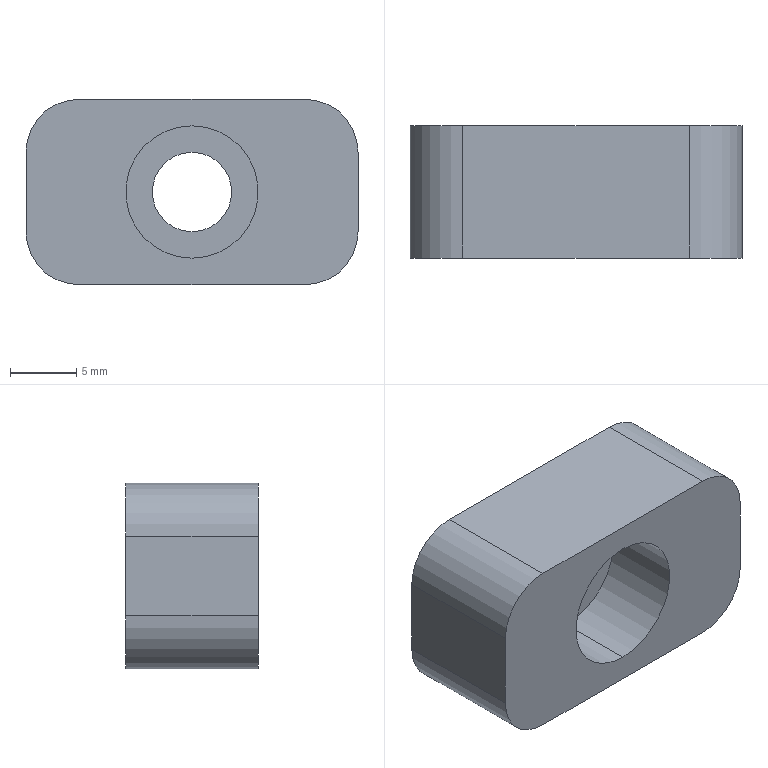Part | STEP file | 1 solid | 15 faces | box 25.075 x 10 x 14 mm | volume 2789 mm3 | cylinder 8 | plane 7 | commonest cylinder face diameters 8 x4 6 x2 10 x2
STEP:
#1=CARTESIAN_POINT('',(0.,0.,0.));
#2=DIRECTION('',(0.,0.,1.));
#3=DIRECTION('',(1.,0.,0.));
#4=AXIS2_PLACEMENT_3D('',#1,#2,#3);
#5=CARTESIAN_POINT('',(-72.862,-50.,192.673));
#6=VERTEX_POINT('',#5);
#7=CARTESIAN_POINT('',(-72.862,-44.,192.673));
#8=VERTEX_POINT('',#7);
#9=CARTESIAN_POINT('',(-72.862,-50.,192.673));
#10=DIRECTION('',(0.,1.,0.));
#11=VECTOR('',#10,1.);
#12=LINE('',#9,#11);
#13=CARTESIAN_POINT('',(-72.862,-50.,187.673));
#14=DIRECTION('',(0.,1.,0.));
#15=DIRECTION('',(0.,0.,1.));
#16=AXIS2_PLACEMENT_3D('',#13,#14,#15);
#17=CYLINDRICAL_SURFACE('',#16,5.);
#18=CARTESIAN_POINT('',(6.283,0.));
#19=DIRECTION('',(0.,1.));
#20=VECTOR('',#19,1.);
#21=LINE('',#18,#20);
#22=(GEOMETRIC_REPRESENTATION_CONTEXT(2)PARAMETRIC_REPRESENTATION_CONTEXT()REPRESENTATION_CONTEXT('',''));
#23=DEFINITIONAL_REPRESENTATION('',(#21),#22);
#24=PCURVE('',#17,#23);
#25=CARTESIAN_POINT('',(-72.862,-50.,187.673));
#26=DIRECTION('',(0.,1.,0.));
#27=DIRECTION('',(0.,0.,1.));
#28=AXIS2_PLACEMENT_3D('',#25,#26,#27);
#29=CYLINDRICAL_SURFACE('',#28,5.);
#30=CARTESIAN_POINT('',(0.,0.));
#31=DIRECTION('',(0.,1.));
#32=VECTOR('',#31,1.);
#33=LINE('',#30,#32);
#34=(GEOMETRIC_REPRESENTATION_CONTEXT(2)PARAMETRIC_REPRESENTATION_CONTEXT()REPRESENTATION_CONTEXT('',''));
#35=DEFINITIONAL_REPRESENTATION('',(#33),#34);
#36=PCURVE('',#29,#35);
#37=SURFACE_CURVE('',#12,(#24,#36),.PCURVE_S1.);
#38=EDGE_CURVE('',#6,#8,#37,.T.);
#39=ORIENTED_EDGE('',*,*,#38,.T.);
#40=CARTESIAN_POINT('',(-72.862,-44.,182.673));
#41=VERTEX_POINT('',#40);
#42=CARTESIAN_POINT('',(-72.862,-44.,187.673));
#43=DIRECTION('',(0.,-1.,0.));
#44=DIRECTION('',(0.,0.,-1.));
#45=AXIS2_PLACEMENT_3D('',#42,#43,#44);
#46=CIRCLE('',#45,5.);
#47=CARTESIAN_POINT('',(9.425,6.));
#48=DIRECTION('',(-1.,0.));
#49=VECTOR('',#48,1.);
#50=LINE('',#47,#49);
#51=(GEOMETRIC_REPRESENTATION_CONTEXT(2)PARAMETRIC_REPRESENTATION_CONTEXT()REPRESENTATION_CONTEXT('',''));
#52=DEFINITIONAL_REPRESENTATION('',(#50),#51);
#53=PCURVE('',#17,#52);
#54=CARTESIAN_POINT('',(-72.862,-44.,187.673));
#55=DIRECTION('',(0.,1.,0.));
#56=DIRECTION('',(0.,0.,1.));
#57=AXIS2_PLACEMENT_3D('',#54,#55,#56);
#58=PLANE('',#57);
#59=CARTESIAN_POINT('',(-5.,0.));
#60=CARTESIAN_POINT('',(-5.,8.66));
#61=CARTESIAN_POINT('',(2.5,4.33));
#62=CARTESIAN_POINT('',(10.,0.));
#63=CARTESIAN_POINT('',(2.5,-4.33));
#64=CARTESIAN_POINT('',(-5.,-8.66));
#65=CARTESIAN_POINT('',(-5.,0.));
#66=(BOUNDED_CURVE()B_SPLINE_CURVE(2,(#59,#60,#61,#62,#63,#64,#65),.UNSPECIFIED.,.T.,.F.)B_SPLINE_CURVE_WITH_KNOTS((1,2,2,2,2,1),(-2.094,0.,2.094,4.189,6.283,8.378),.UNSPECIFIED.)CURVE()GEOMETRIC_REPRESENTATION_ITEM()RATIONAL_B_SPLINE_CURVE((1.,0.5,1.,0.5,1.,0.5,1.))REPRESENTATION_ITEM(''));
#67=(GEOMETRIC_REPRESENTATION_CONTEXT(2)PARAMETRIC_REPRESENTATION_CONTEXT()REPRESENTATION_CONTEXT('',''));
#68=DEFINITIONAL_REPRESENTATION('',(#66),#67);
#69=PCURVE('',#58,#68);
#70=SURFACE_CURVE('',#46,(#53,#69),.PCURVE_S1.);
#71=EDGE_CURVE('',#8,#41,#70,.T.);
#72=ORIENTED_EDGE('',*,*,#71,.T.);
#73=CARTESIAN_POINT('',(-72.862,-50.,182.673));
#74=VERTEX_POINT('',#73);
#75=CARTESIAN_POINT('',(-72.862,-50.,182.673));
#76=DIRECTION('',(0.,1.,0.));
#77=VECTOR('',#76,1.);
#78=LINE('',#75,#77);
#79=CARTESIAN_POINT('',(3.142,0.));
#80=DIRECTION('',(0.,1.));
#81=VECTOR('',#80,1.);
#82=LINE('',#79,#81);
#83=(GEOMETRIC_REPRESENTATION_CONTEXT(2)PARAMETRIC_REPRESENTATION_CONTEXT()REPRESENTATION_CONTEXT('',''));
#84=DEFINITIONAL_REPRESENTATION('',(#82),#83);
#85=PCURVE('',#17,#84);
#86=CARTESIAN_POINT('',(3.142,0.));
#87=DIRECTION('',(0.,1.));
#88=VECTOR('',#87,1.);
#89=LINE('',#86,#88);
#90=(GEOMETRIC_REPRESENTATION_CONTEXT(2)PARAMETRIC_REPRESENTATION_CONTEXT()REPRESENTATION_CONTEXT('',''));
#91=DEFINITIONAL_REPRESENTATION('',(#89),#90);
#92=PCURVE('',#29,#91);
#93=SURFACE_CURVE('',#78,(#85,#92),.PCURVE_S1.);
#94=EDGE_CURVE('',#74,#41,#93,.T.);
#95=ORIENTED_EDGE('',*,*,#94,.F.);
#96=CARTESIAN_POINT('',(-72.862,-50.,187.673));
#97=DIRECTION('',(0.,1.,0.));
#98=DIRECTION('',(0.,0.,1.));
#99=AXIS2_PLACEMENT_3D('',#96,#97,#98);
#100=CIRCLE('',#99,5.);
#101=CARTESIAN_POINT('',(0.,0.));
#102=DIRECTION('',(1.,0.));
#103=VECTOR('',#102,1.);
#104=LINE('',#101,#103);
#105=(GEOMETRIC_REPRESENTATION_CONTEXT(2)PARAMETRIC_REPRESENTATION_CONTEXT()REPRESENTATION_CONTEXT('',''));
#106=DEFINITIONAL_REPRESENTATION('',(#104),#105);
#107=PCURVE('',#17,#106);
#108=CARTESIAN_POINT('',(-72.862,-50.,180.923));
#109=DIRECTION('',(0.,-1.,0.));
#110=DIRECTION('',(0.,0.,-1.));
#111=AXIS2_PLACEMENT_3D('',#108,#109,#110);
#112=PLANE('',#111);
#113=CARTESIAN_POINT('',(-11.75,0.));
#114=CARTESIAN_POINT('',(-11.75,8.66));
#115=CARTESIAN_POINT('',(-4.25,4.33));
#116=CARTESIAN_POINT('',(3.25,0.));
#117=CARTESIAN_POINT('',(-4.25,-4.33));
#118=CARTESIAN_POINT('',(-11.75,-8.66));
#119=CARTESIAN_POINT('',(-11.75,0.));
#120=(BOUNDED_CURVE()B_SPLINE_CURVE(2,(#113,#114,#115,#116,#117,#118,#119),.UNSPECIFIED.,.T.,.F.)B_SPLINE_CURVE_WITH_KNOTS((1,2,2,2,2,1),(-2.094,0.,2.094,4.189,6.283,8.378),.UNSPECIFIED.)CURVE()GEOMETRIC_REPRESENTATION_ITEM()RATIONAL_B_SPLINE_CURVE((1.,0.5,1.,0.5,1.,0.5,1.))REPRESENTATION_ITEM(''));
#121=(GEOMETRIC_REPRESENTATION_CONTEXT(2)PARAMETRIC_REPRESENTATION_CONTEXT()REPRESENTATION_CONTEXT('',''));
#122=DEFINITIONAL_REPRESENTATION('',(#120),#121);
#123=PCURVE('',#112,#122);
#124=SURFACE_CURVE('',#100,(#107,#123),.PCURVE_S1.);
#125=EDGE_CURVE('',#74,#6,#124,.T.);
#126=ORIENTED_EDGE('',*,*,#125,.T.);
#127=EDGE_LOOP('',(#39,#72,#95,#126));
#128=FACE_BOUND('',#127,.F.);
#129=ADVANCED_FACE('',(#128),#17,.F.);
#130=CARTESIAN_POINT('',(-72.862,-44.,190.673));
#131=VERTEX_POINT('',#130);
#132=CARTESIAN_POINT('',(-72.862,-40.,190.673));
#133=VERTEX_POINT('',#132);
#134=CARTESIAN_POINT('',(-72.862,-50.,190.673));
#135=DIRECTION('',(0.,1.,0.));
#136=VECTOR('',#135,1.);
#137=LINE('',#134,#136);
#138=CARTESIAN_POINT('',(-72.862,-50.,187.673));
#139=DIRECTION('',(0.,1.,0.));
#140=DIRECTION('',(0.,0.,1.));
#141=AXIS2_PLACEMENT_3D('',#138,#139,#140);
#142=CYLINDRICAL_SURFACE('',#141,3.);
#143=CARTESIAN_POINT('',(6.283,0.));
#144=DIRECTION('',(0.,1.));
#145=VECTOR('',#144,1.);
#146=LINE('',#143,#145);
#147=(GEOMETRIC_REPRESENTATION_CONTEXT(2)PARAMETRIC_REPRESENTATION_CONTEXT()REPRESENTATION_CONTEXT('',''));
#148=DEFINITIONAL_REPRESENTATION('',(#146),#147);
#149=PCURVE('',#142,#148);
#150=CARTESIAN_POINT('',(-72.862,-50.,187.673));
#151=DIRECTION('',(0.,1.,0.));
#152=DIRECTION('',(0.,0.,1.));
#153=AXIS2_PLACEMENT_3D('',#150,#151,#152);
#154=CYLINDRICAL_SURFACE('',#153,3.);
#155=CARTESIAN_POINT('',(0.,0.));
#156=DIRECTION('',(0.,1.));
#157=VECTOR('',#156,1.);
#158=LINE('',#155,#157);
#159=(GEOMETRIC_REPRESENTATION_CONTEXT(2)PARAMETRIC_REPRESENTATION_CONTEXT()REPRESENTATION_CONTEXT('',''));
#160=DEFINITIONAL_REPRESENTATION('',(#158),#159);
#161=PCURVE('',#154,#160);
#162=SURFACE_CURVE('',#137,(#149,#161),.PCURVE_S1.);
#163=EDGE_CURVE('',#131,#133,#162,.T.);
#164=ORIENTED_EDGE('',*,*,#163,.T.);
#165=CARTESIAN_POINT('',(-72.862,-40.,184.673));
#166=VERTEX_POINT('',#165);
#167=CARTESIAN_POINT('',(-72.862,-40.,187.673));
#168=DIRECTION('',(0.,-1.,0.));
#169=DIRECTION('',(0.,0.,-1.));
#170=AXIS2_PLACEMENT_3D('',#167,#168,#169);
#171=CIRCLE('',#170,3.);
#172=CARTESIAN_POINT('',(9.425,10.));
#173=DIRECTION('',(-1.,0.));
#174=VECTOR('',#173,1.);
#175=LINE('',#172,#174);
#176=(GEOMETRIC_REPRESENTATION_CONTEXT(2)PARAMETRIC_REPRESENTATION_CONTEXT()REPRESENTATION_CONTEXT('',''));
#177=DEFINITIONAL_REPRESENTATION('',(#175),#176);
#178=PCURVE('',#142,#177);
#179=CARTESIAN_POINT('',(-72.862,-40.,187.923));
#180=DIRECTION('',(0.,-1.,0.));
#181=DIRECTION('',(0.,0.,-1.));
#182=AXIS2_PLACEMENT_3D('',#179,#180,#181);
#183=PLANE('',#182);
#184=CARTESIAN_POINT('',(0.25,0.));
#185=DIRECTION('',(1.,0.));
#186=AXIS2_PLACEMENT_2D('',#184,#185);
#187=CIRCLE('',#186,3.);
#188=(GEOMETRIC_REPRESENTATION_CONTEXT(2)PARAMETRIC_REPRESENTATION_CONTEXT()REPRESENTATION_CONTEXT('',''));
#189=DEFINITIONAL_REPRESENTATION('',(#187),#188);
#190=PCURVE('',#183,#189);
#191=SURFACE_CURVE('',#171,(#178,#190),.PCURVE_S1.);
#192=EDGE_CURVE('',#133,#166,#191,.T.);
#193=ORIENTED_EDGE('',*,*,#192,.T.);
#194=CARTESIAN_POINT('',(-72.862,-44.,184.673));
#195=VERTEX_POINT('',#194);
#196=CARTESIAN_POINT('',(-72.862,-50.,184.673));
#197=DIRECTION('',(0.,1.,0.));
#198=VECTOR('',#197,1.);
#199=LINE('',#196,#198);
#200=CARTESIAN_POINT('',(3.142,0.));
#201=DIRECTION('',(0.,1.));
#202=VECTOR('',#201,1.);
#203=LINE('',#200,#202);
#204=(GEOMETRIC_REPRESENTATION_CONTEXT(2)PARAMETRIC_REPRESENTATION_CONTEXT()REPRESENTATION_CONTEXT('',''));
#205=DEFINITIONAL_REPRESENTATION('',(#203),#204);
#206=PCURVE('',#142,#205);
#207=CARTESIAN_POINT('',(3.142,0.));
#208=DIRECTION('',(0.,1.));
#209=VECTOR('',#208,1.);
#210=LINE('',#207,#209);
#211=(GEOMETRIC_REPRESENTATION_CONTEXT(2)PARAMETRIC_REPRESENTATION_CONTEXT()REPRESENTATION_CONTEXT('',''));
#212=DEFINITIONAL_REPRESENTATION('',(#210),#211);
#213=PCURVE('',#154,#212);
#214=SURFACE_CURVE('',#199,(#206,#213),.PCURVE_S1.);
#215=EDGE_CURVE('',#195,#166,#214,.T.);
#216=ORIENTED_EDGE('',*,*,#215,.F.);
#217=CARTESIAN_POINT('',(-72.862,-44.,187.673));
#218=DIRECTION('',(0.,-1.,0.));
#219=DIRECTION('',(0.,0.,1.));
#220=AXIS2_PLACEMENT_3D('',#217,#218,#219);
#221=CIRCLE('',#220,3.);
#222=CARTESIAN_POINT('',(6.283,6.));
#223=DIRECTION('',(-1.,0.));
#224=VECTOR('',#223,1.);
#225=LINE('',#222,#224);
#226=(GEOMETRIC_REPRESENTATION_CONTEXT(2)PARAMETRIC_REPRESENTATION_CONTEXT()REPRESENTATION_CONTEXT('',''));
#227=DEFINITIONAL_REPRESENTATION('',(#225),#226);
#228=PCURVE('',#142,#227);
#229=CARTESIAN_POINT('',(3.,0.));
#230=CARTESIAN_POINT('',(3.,-5.196));
#231=CARTESIAN_POINT('',(-1.5,-2.598));
#232=CARTESIAN_POINT('',(-6.,0.));
#233=CARTESIAN_POINT('',(-1.5,2.598));
#234=CARTESIAN_POINT('',(3.,5.196));
#235=CARTESIAN_POINT('',(3.,0.));
#236=(BOUNDED_CURVE()B_SPLINE_CURVE(2,(#229,#230,#231,#232,#233,#234,#235),.UNSPECIFIED.,.T.,.F.)B_SPLINE_CURVE_WITH_KNOTS((1,2,2,2,2,1),(-2.094,0.,2.094,4.189,6.283,8.378),.UNSPECIFIED.)CURVE()GEOMETRIC_REPRESENTATION_ITEM()RATIONAL_B_SPLINE_CURVE((1.,0.5,1.,0.5,1.,0.5,1.))REPRESENTATION_ITEM(''));
#237=(GEOMETRIC_REPRESENTATION_CONTEXT(2)PARAMETRIC_REPRESENTATION_CONTEXT()REPRESENTATION_CONTEXT('',''));
#238=DEFINITIONAL_REPRESENTATION('',(#236),#237);
#239=PCURVE('',#58,#238);
#240=SURFACE_CURVE('',#221,(#228,#239),.PCURVE_S1.);
#241=EDGE_CURVE('',#131,#195,#240,.T.);
#242=ORIENTED_EDGE('',*,*,#241,.F.);
#243=EDGE_LOOP('',(#164,#193,#216,#242));
#244=FACE_BOUND('',#243,.F.);
#245=ADVANCED_FACE('',(#244),#142,.F.);
#246=CARTESIAN_POINT('',(-81.4,-50.,180.673));
#247=VERTEX_POINT('',#246);
#248=CARTESIAN_POINT('',(-64.325,-50.,180.673));
#249=VERTEX_POINT('',#248);
#250=CARTESIAN_POINT('',(-72.862,-50.,180.673));
#251=DIRECTION('',(1.,0.,0.));
#252=VECTOR('',#251,1.);
#253=LINE('',#250,#252);
#254=CARTESIAN_POINT('',(-72.862,-42.,180.673));
#255=DIRECTION('',(0.,0.,-1.));
#256=DIRECTION('',(-1.,0.,0.));
#257=AXIS2_PLACEMENT_3D('',#254,#255,#256);
#258=PLANE('',#257);
#259=CARTESIAN_POINT('',(0.,-8.));
#260=DIRECTION('',(-1.,0.));
#261=VECTOR('',#260,1.);
#262=LINE('',#259,#261);
#263=(GEOMETRIC_REPRESENTATION_CONTEXT(2)PARAMETRIC_REPRESENTATION_CONTEXT()REPRESENTATION_CONTEXT('',''));
#264=DEFINITIONAL_REPRESENTATION('',(#262),#263);
#265=PCURVE('',#258,#264);
#266=CARTESIAN_POINT('',(0.25,0.));
#267=DIRECTION('',(0.,1.));
#268=VECTOR('',#267,1.);
#269=LINE('',#266,#268);
#270=(GEOMETRIC_REPRESENTATION_CONTEXT(2)PARAMETRIC_REPRESENTATION_CONTEXT()REPRESENTATION_CONTEXT('',''));
#271=DEFINITIONAL_REPRESENTATION('',(#269),#270);
#272=PCURVE('',#112,#271);
#273=SURFACE_CURVE('',#253,(#265,#272),.PCURVE_S1.);
#274=EDGE_CURVE('',#247,#249,#273,.T.);
#275=ORIENTED_EDGE('',*,*,#274,.F.);
#276=CARTESIAN_POINT('',(-81.4,-40.,180.673));
#277=VERTEX_POINT('',#276);
#278=CARTESIAN_POINT('',(-81.4,-42.,180.673));
#279=DIRECTION('',(0.,1.,0.));
#280=VECTOR('',#279,1.);
#281=LINE('',#278,#280);
#282=CARTESIAN_POINT('',(8.537,0.));
#283=DIRECTION('',(0.,1.));
#284=VECTOR('',#283,1.);
#285=LINE('',#282,#284);
#286=(GEOMETRIC_REPRESENTATION_CONTEXT(2)PARAMETRIC_REPRESENTATION_CONTEXT()REPRESENTATION_CONTEXT('',''));
#287=DEFINITIONAL_REPRESENTATION('',(#285),#286);
#288=PCURVE('',#258,#287);
#289=CARTESIAN_POINT('',(-81.4,-42.,184.673));
#290=DIRECTION('',(0.,-1.,0.));
#291=DIRECTION('',(0.,0.,-1.));
#292=AXIS2_PLACEMENT_3D('',#289,#290,#291);
#293=CYLINDRICAL_SURFACE('',#292,4.);
#294=CARTESIAN_POINT('',(6.283,0.));
#295=DIRECTION('',(0.,-1.));
#296=VECTOR('',#295,1.);
#297=LINE('',#294,#296);
#298=(GEOMETRIC_REPRESENTATION_CONTEXT(2)PARAMETRIC_REPRESENTATION_CONTEXT()REPRESENTATION_CONTEXT('',''));
#299=DEFINITIONAL_REPRESENTATION('',(#297),#298);
#300=PCURVE('',#293,#299);
#301=SURFACE_CURVE('',#281,(#288,#300),.PCURVE_S1.);
#302=EDGE_CURVE('',#247,#277,#301,.T.);
#303=ORIENTED_EDGE('',*,*,#302,.T.);
#304=CARTESIAN_POINT('',(-64.325,-40.,180.673));
#305=VERTEX_POINT('',#304);
#306=CARTESIAN_POINT('',(-72.862,-40.,180.673));
#307=DIRECTION('',(-1.,0.,0.));
#308=VECTOR('',#307,1.);
#309=LINE('',#306,#308);
#310=CARTESIAN_POINT('',(0.,2.));
#311=DIRECTION('',(1.,0.));
#312=VECTOR('',#311,1.);
#313=LINE('',#310,#312);
#314=(GEOMETRIC_REPRESENTATION_CONTEXT(2)PARAMETRIC_REPRESENTATION_CONTEXT()REPRESENTATION_CONTEXT('',''));
#315=DEFINITIONAL_REPRESENTATION('',(#313),#314);
#316=PCURVE('',#258,#315);
#317=CARTESIAN_POINT('',(7.25,0.));
#318=DIRECTION('',(0.,-1.));
#319=VECTOR('',#318,1.);
#320=LINE('',#317,#319);
#321=(GEOMETRIC_REPRESENTATION_CONTEXT(2)PARAMETRIC_REPRESENTATION_CONTEXT()REPRESENTATION_CONTEXT('',''));
#322=DEFINITIONAL_REPRESENTATION('',(#320),#321);
#323=PCURVE('',#183,#322);
#324=SURFACE_CURVE('',#309,(#316,#323),.PCURVE_S1.);
#325=EDGE_CURVE('',#305,#277,#324,.T.);
#326=ORIENTED_EDGE('',*,*,#325,.F.);
#327=CARTESIAN_POINT('',(-64.325,-42.,180.673));
#328=DIRECTION('',(0.,-1.,0.));
#329=VECTOR('',#328,1.);
#330=LINE('',#327,#329);
#331=CARTESIAN_POINT('',(-8.537,0.));
#332=DIRECTION('',(0.,-1.));
#333=VECTOR('',#332,1.);
#334=LINE('',#331,#333);
#335=(GEOMETRIC_REPRESENTATION_CONTEXT(2)PARAMETRIC_REPRESENTATION_CONTEXT()REPRESENTATION_CONTEXT('',''));
#336=DEFINITIONAL_REPRESENTATION('',(#334),#335);
#337=PCURVE('',#258,#336);
#338=CARTESIAN_POINT('',(-64.325,-42.,184.673));
#339=DIRECTION('',(0.,1.,0.));
#340=DIRECTION('',(0.,0.,1.));
#341=AXIS2_PLACEMENT_3D('',#338,#339,#340);
#342=CYLINDRICAL_SURFACE('',#341,4.);
#343=CARTESIAN_POINT('',(3.142,0.));
#344=DIRECTION('',(0.,-1.));
#345=VECTOR('',#344,1.);
#346=LINE('',#343,#345);
#347=(GEOMETRIC_REPRESENTATION_CONTEXT(2)PARAMETRIC_REPRESENTATION_CONTEXT()REPRESENTATION_CONTEXT('',''));
#348=DEFINITIONAL_REPRESENTATION('',(#346),#347);
#349=PCURVE('',#342,#348);
#350=SURFACE_CURVE('',#330,(#337,#349),.PCURVE_S1.);
#351=EDGE_CURVE('',#305,#249,#350,.T.);
#352=ORIENTED_EDGE('',*,*,#351,.T.);
#353=EDGE_LOOP('',(#275,#303,#326,#352));
#354=FACE_BOUND('',#353,.T.);
#355=ADVANCED_FACE('',(#354),#258,.T.);
#356=ORIENTED_EDGE('',*,*,#192,.T.);
#357=CARTESIAN_POINT('',(-72.862,-40.,187.673));
#358=DIRECTION('',(0.,-1.,0.));
#359=DIRECTION('',(0.,0.,-1.));
#360=AXIS2_PLACEMENT_3D('',#357,#358,#359);
#361=CIRCLE('',#360,3.);
#362=CARTESIAN_POINT('',(0.25,0.));
#363=DIRECTION('',(1.,0.));
#364=AXIS2_PLACEMENT_2D('',#362,#363);
#365=CIRCLE('',#364,3.);
#366=(GEOMETRIC_REPRESENTATION_CONTEXT(2)PARAMETRIC_REPRESENTATION_CONTEXT()REPRESENTATION_CONTEXT('',''));
#367=DEFINITIONAL_REPRESENTATION('',(#365),#366);
#368=PCURVE('',#183,#367);
#369=CARTESIAN_POINT('',(3.142,10.));
#370=DIRECTION('',(-1.,0.));
#371=VECTOR('',#370,1.);
#372=LINE('',#369,#371);
#373=(GEOMETRIC_REPRESENTATION_CONTEXT(2)PARAMETRIC_REPRESENTATION_CONTEXT()REPRESENTATION_CONTEXT('',''));
#374=DEFINITIONAL_REPRESENTATION('',(#372),#373);
#375=PCURVE('',#154,#374);
#376=SURFACE_CURVE('',#361,(#368,#375),.PCURVE_S1.);
#377=EDGE_CURVE('',#166,#133,#376,.T.);
#378=ORIENTED_EDGE('',*,*,#377,.T.);
#379=EDGE_LOOP('',(#356,#378));
#380=FACE_BOUND('',#379,.T.);
#381=ORIENTED_EDGE('',*,*,#325,.T.);
#382=CARTESIAN_POINT('',(-85.4,-40.,184.673));
#383=VERTEX_POINT('',#382);
#384=CARTESIAN_POINT('',(-81.4,-40.,184.673));
#385=DIRECTION('',(0.,1.,0.));
#386=DIRECTION('',(0.,0.,-1.));
#387=AXIS2_PLACEMENT_3D('',#384,#385,#386);
#388=CIRCLE('',#387,4.);
#389=CARTESIAN_POINT('',(7.25,-8.537));
#390=CARTESIAN_POINT('',(7.25,-15.466));
#391=CARTESIAN_POINT('',(1.25,-12.002));
#392=CARTESIAN_POINT('',(-4.75,-8.537));
#393=CARTESIAN_POINT('',(1.25,-5.073));
#394=CARTESIAN_POINT('',(7.25,-1.609));
#395=CARTESIAN_POINT('',(7.25,-8.537));
#396=(BOUNDED_CURVE()B_SPLINE_CURVE(2,(#389,#390,#391,#392,#393,#394,#395),.UNSPECIFIED.,.T.,.F.)B_SPLINE_CURVE_WITH_KNOTS((1,2,2,2,2,1),(-2.094,0.,2.094,4.189,6.283,8.378),.UNSPECIFIED.)CURVE()GEOMETRIC_REPRESENTATION_ITEM()RATIONAL_B_SPLINE_CURVE((1.,0.5,1.,0.5,1.,0.5,1.))REPRESENTATION_ITEM(''));
#397=(GEOMETRIC_REPRESENTATION_CONTEXT(2)PARAMETRIC_REPRESENTATION_CONTEXT()REPRESENTATION_CONTEXT('',''));
#398=DEFINITIONAL_REPRESENTATION('',(#396),#397);
#399=PCURVE('',#183,#398);
#400=CARTESIAN_POINT('',(6.283,-2.));
#401=DIRECTION('',(-1.,0.));
#402=VECTOR('',#401,1.);
#403=LINE('',#400,#402);
#404=(GEOMETRIC_REPRESENTATION_CONTEXT(2)PARAMETRIC_REPRESENTATION_CONTEXT()REPRESENTATION_CONTEXT('',''));
#405=DEFINITIONAL_REPRESENTATION('',(#403),#404);
#406=PCURVE('',#293,#405);
#407=SURFACE_CURVE('',#388,(#399,#406),.PCURVE_S1.);
#408=EDGE_CURVE('',#277,#383,#407,.T.);
#409=ORIENTED_EDGE('',*,*,#408,.T.);
#410=CARTESIAN_POINT('',(-85.4,-40.,190.673));
#411=VERTEX_POINT('',#410);
#412=CARTESIAN_POINT('',(-85.4,-40.,180.923));
#413=DIRECTION('',(0.,0.,1.));
#414=VECTOR('',#413,1.);
#415=LINE('',#412,#414);
#416=CARTESIAN_POINT('',(7.,-12.537));
#417=DIRECTION('',(-1.,0.));
#418=VECTOR('',#417,1.);
#419=LINE('',#416,#418);
#420=(GEOMETRIC_REPRESENTATION_CONTEXT(2)PARAMETRIC_REPRESENTATION_CONTEXT()REPRESENTATION_CONTEXT('',''));
#421=DEFINITIONAL_REPRESENTATION('',(#419),#420);
#422=PCURVE('',#183,#421);
#423=CARTESIAN_POINT('',(-85.4,-42.,180.923));
#424=DIRECTION('',(-1.,0.,0.));
#425=DIRECTION('',(0.,0.,1.));
#426=AXIS2_PLACEMENT_3D('',#423,#424,#425);
#427=PLANE('',#426);
#428=CARTESIAN_POINT('',(0.,2.));
#429=DIRECTION('',(1.,0.));
#430=VECTOR('',#429,1.);
#431=LINE('',#428,#430);
#432=(GEOMETRIC_REPRESENTATION_CONTEXT(2)PARAMETRIC_REPRESENTATION_CONTEXT()REPRESENTATION_CONTEXT('',''));
#433=DEFINITIONAL_REPRESENTATION('',(#431),#432);
#434=PCURVE('',#427,#433);
#435=SURFACE_CURVE('',#415,(#422,#434),.PCURVE_S1.);
#436=EDGE_CURVE('',#383,#411,#435,.T.);
#437=ORIENTED_EDGE('',*,*,#436,.T.);
#438=CARTESIAN_POINT('',(-81.4,-40.,194.673));
#439=VERTEX_POINT('',#438);
#440=CARTESIAN_POINT('',(-81.4,-40.,190.673));
#441=DIRECTION('',(0.,1.,0.));
#442=DIRECTION('',(0.,0.,-1.));
#443=AXIS2_PLACEMENT_3D('',#440,#441,#442);
#444=CIRCLE('',#443,4.);
#445=CARTESIAN_POINT('',(1.25,-8.537));
#446=CARTESIAN_POINT('',(1.25,-15.466));
#447=CARTESIAN_POINT('',(-4.75,-12.002));
#448=CARTESIAN_POINT('',(-10.75,-8.537));
#449=CARTESIAN_POINT('',(-4.75,-5.073));
#450=CARTESIAN_POINT('',(1.25,-1.609));
#451=CARTESIAN_POINT('',(1.25,-8.537));
#452=(BOUNDED_CURVE()B_SPLINE_CURVE(2,(#445,#446,#447,#448,#449,#450,#451),.UNSPECIFIED.,.T.,.F.)B_SPLINE_CURVE_WITH_KNOTS((1,2,2,2,2,1),(-2.094,0.,2.094,4.189,6.283,8.378),.UNSPECIFIED.)CURVE()GEOMETRIC_REPRESENTATION_ITEM()RATIONAL_B_SPLINE_CURVE((1.,0.5,1.,0.5,1.,0.5,1.))REPRESENTATION_ITEM(''));
#453=(GEOMETRIC_REPRESENTATION_CONTEXT(2)PARAMETRIC_REPRESENTATION_CONTEXT()REPRESENTATION_CONTEXT('',''));
#454=DEFINITIONAL_REPRESENTATION('',(#452),#453);
#455=PCURVE('',#183,#454);
#456=CARTESIAN_POINT('',(-81.4,-45.,190.673));
#457=DIRECTION('',(0.,1.,0.));
#458=DIRECTION('',(0.,0.,1.));
#459=AXIS2_PLACEMENT_3D('',#456,#457,#458);
#460=CYLINDRICAL_SURFACE('',#459,4.);
#461=CARTESIAN_POINT('',(3.142,5.));
#462=DIRECTION('',(1.,0.));
#463=VECTOR('',#462,1.);
#464=LINE('',#461,#463);
#465=(GEOMETRIC_REPRESENTATION_CONTEXT(2)PARAMETRIC_REPRESENTATION_CONTEXT()REPRESENTATION_CONTEXT('',''));
#466=DEFINITIONAL_REPRESENTATION('',(#464),#465);
#467=PCURVE('',#460,#466);
#468=SURFACE_CURVE('',#444,(#455,#467),.PCURVE_S1.);
#469=EDGE_CURVE('',#411,#439,#468,.T.);
#470=ORIENTED_EDGE('',*,*,#469,.T.);
#471=CARTESIAN_POINT('',(-64.325,-40.,194.673));
#472=VERTEX_POINT('',#471);
#473=CARTESIAN_POINT('',(-72.862,-40.,194.673));
#474=DIRECTION('',(1.,0.,0.));
#475=VECTOR('',#474,1.);
#476=LINE('',#473,#475);
#477=CARTESIAN_POINT('',(-6.75,0.));
#478=DIRECTION('',(0.,1.));
#479=VECTOR('',#478,1.);
#480=LINE('',#477,#479);
#481=(GEOMETRIC_REPRESENTATION_CONTEXT(2)PARAMETRIC_REPRESENTATION_CONTEXT()REPRESENTATION_CONTEXT('',''));
#482=DEFINITIONAL_REPRESENTATION('',(#480),#481);
#483=PCURVE('',#183,#482);
#484=CARTESIAN_POINT('',(-72.862,-45.,194.673));
#485=DIRECTION('',(0.,0.,-1.));
#486=DIRECTION('',(-1.,0.,0.));
#487=AXIS2_PLACEMENT_3D('',#484,#485,#486);
#488=PLANE('',#487);
#489=CARTESIAN_POINT('',(0.,5.));
#490=DIRECTION('',(-1.,0.));
#491=VECTOR('',#490,1.);
#492=LINE('',#489,#491);
#493=(GEOMETRIC_REPRESENTATION_CONTEXT(2)PARAMETRIC_REPRESENTATION_CONTEXT()REPRESENTATION_CONTEXT('',''));
#494=DEFINITIONAL_REPRESENTATION('',(#492),#493);
#495=PCURVE('',#488,#494);
#496=SURFACE_CURVE('',#476,(#483,#495),.PCURVE_S1.);
#497=EDGE_CURVE('',#439,#472,#496,.T.);
#498=ORIENTED_EDGE('',*,*,#497,.T.);
#499=CARTESIAN_POINT('',(-60.325,-40.,190.673));
#500=VERTEX_POINT('',#499);
#501=CARTESIAN_POINT('',(-64.325,-40.,190.673));
#502=DIRECTION('',(0.,1.,0.));
#503=DIRECTION('',(0.,0.,-1.));
#504=AXIS2_PLACEMENT_3D('',#501,#502,#503);
#505=CIRCLE('',#504,4.);
#506=CARTESIAN_POINT('',(1.25,8.537));
#507=CARTESIAN_POINT('',(1.25,1.609));
#508=CARTESIAN_POINT('',(-4.75,5.073));
#509=CARTESIAN_POINT('',(-10.75,8.537));
#510=CARTESIAN_POINT('',(-4.75,12.002));
#511=CARTESIAN_POINT('',(1.25,15.466));
#512=CARTESIAN_POINT('',(1.25,8.537));
#513=(BOUNDED_CURVE()B_SPLINE_CURVE(2,(#506,#507,#508,#509,#510,#511,#512),.UNSPECIFIED.,.T.,.F.)B_SPLINE_CURVE_WITH_KNOTS((1,2,2,2,2,1),(-2.094,0.,2.094,4.189,6.283,8.378),.UNSPECIFIED.)CURVE()GEOMETRIC_REPRESENTATION_ITEM()RATIONAL_B_SPLINE_CURVE((1.,0.5,1.,0.5,1.,0.5,1.))REPRESENTATION_ITEM(''));
#514=(GEOMETRIC_REPRESENTATION_CONTEXT(2)PARAMETRIC_REPRESENTATION_CONTEXT()REPRESENTATION_CONTEXT('',''));
#515=DEFINITIONAL_REPRESENTATION('',(#513),#514);
#516=PCURVE('',#183,#515);
#517=CARTESIAN_POINT('',(-64.325,-45.,190.673));
#518=DIRECTION('',(0.,-1.,0.));
#519=DIRECTION('',(0.,0.,-1.));
#520=AXIS2_PLACEMENT_3D('',#517,#518,#519);
#521=CYLINDRICAL_SURFACE('',#520,4.);
#522=CARTESIAN_POINT('',(6.283,-5.));
#523=DIRECTION('',(-1.,0.));
#524=VECTOR('',#523,1.);
#525=LINE('',#522,#524);
#526=(GEOMETRIC_REPRESENTATION_CONTEXT(2)PARAMETRIC_REPRESENTATION_CONTEXT()REPRESENTATION_CONTEXT('',''));
#527=DEFINITIONAL_REPRESENTATION('',(#525),#526);
#528=PCURVE('',#521,#527);
#529=SURFACE_CURVE('',#505,(#516,#528),.PCURVE_S1.);
#530=EDGE_CURVE('',#472,#500,#529,.T.);
#531=ORIENTED_EDGE('',*,*,#530,.T.);
#532=CARTESIAN_POINT('',(-60.325,-40.,184.673));
#533=VERTEX_POINT('',#532);
#534=CARTESIAN_POINT('',(-60.325,-40.,180.923));
#535=DIRECTION('',(0.,0.,-1.));
#536=VECTOR('',#535,1.);
#537=LINE('',#534,#536);
#538=CARTESIAN_POINT('',(7.,12.537));
#539=DIRECTION('',(1.,0.));
#540=VECTOR('',#539,1.);
#541=LINE('',#538,#540);
#542=(GEOMETRIC_REPRESENTATION_CONTEXT(2)PARAMETRIC_REPRESENTATION_CONTEXT()REPRESENTATION_CONTEXT('',''));
#543=DEFINITIONAL_REPRESENTATION('',(#541),#542);
#544=PCURVE('',#183,#543);
#545=CARTESIAN_POINT('',(-60.325,-42.,180.923));
#546=DIRECTION('',(1.,0.,0.));
#547=DIRECTION('',(0.,0.,-1.));
#548=AXIS2_PLACEMENT_3D('',#545,#546,#547);
#549=PLANE('',#548);
#550=CARTESIAN_POINT('',(0.,2.));
#551=DIRECTION('',(1.,0.));
#552=VECTOR('',#551,1.);
#553=LINE('',#550,#552);
#554=(GEOMETRIC_REPRESENTATION_CONTEXT(2)PARAMETRIC_REPRESENTATION_CONTEXT()REPRESENTATION_CONTEXT('',''));
#555=DEFINITIONAL_REPRESENTATION('',(#553),#554);
#556=PCURVE('',#549,#555);
#557=SURFACE_CURVE('',#537,(#544,#556),.PCURVE_S1.);
#558=EDGE_CURVE('',#500,#533,#557,.T.);
#559=ORIENTED_EDGE('',*,*,#558,.T.);
#560=CARTESIAN_POINT('',(-64.325,-40.,184.673));
#561=DIRECTION('',(0.,1.,0.));
#562=DIRECTION('',(0.,0.,-1.));
#563=AXIS2_PLACEMENT_3D('',#560,#561,#562);
#564=CIRCLE('',#563,4.);
#565=CARTESIAN_POINT('',(7.25,8.537));
#566=CARTESIAN_POINT('',(7.25,1.609));
#567=CARTESIAN_POINT('',(1.25,5.073));
#568=CARTESIAN_POINT('',(-4.75,8.537));
#569=CARTESIAN_POINT('',(1.25,12.002));
#570=CARTESIAN_POINT('',(7.25,15.466));
#571=CARTESIAN_POINT('',(7.25,8.537));
#572=(BOUNDED_CURVE()B_SPLINE_CURVE(2,(#565,#566,#567,#568,#569,#570,#571),.UNSPECIFIED.,.T.,.F.)B_SPLINE_CURVE_WITH_KNOTS((1,2,2,2,2,1),(-2.094,0.,2.094,4.189,6.283,8.378),.UNSPECIFIED.)CURVE()GEOMETRIC_REPRESENTATION_ITEM()RATIONAL_B_SPLINE_CURVE((1.,0.5,1.,0.5,1.,0.5,1.))REPRESENTATION_ITEM(''));
#573=(GEOMETRIC_REPRESENTATION_CONTEXT(2)PARAMETRIC_REPRESENTATION_CONTEXT()REPRESENTATION_CONTEXT('',''));
#574=DEFINITIONAL_REPRESENTATION('',(#572),#573);
#575=PCURVE('',#183,#574);
#576=CARTESIAN_POINT('',(-3.142,2.));
#577=DIRECTION('',(1.,0.));
#578=VECTOR('',#577,1.);
#579=LINE('',#576,#578);
#580=(GEOMETRIC_REPRESENTATION_CONTEXT(2)PARAMETRIC_REPRESENTATION_CONTEXT()REPRESENTATION_CONTEXT('',''));
#581=DEFINITIONAL_REPRESENTATION('',(#579),#580);
#582=PCURVE('',#342,#581);
#583=SURFACE_CURVE('',#564,(#575,#582),.PCURVE_S1.);
#584=EDGE_CURVE('',#533,#305,#583,.T.);
#585=ORIENTED_EDGE('',*,*,#584,.T.);
#586=EDGE_LOOP('',(#381,#409,#437,#470,#498,#531,#559,#585));
#587=FACE_BOUND('',#586,.T.);
#588=ADVANCED_FACE('',(#380,#587),#183,.F.);
#589=CARTESIAN_POINT('',(-60.325,-50.,184.673));
#590=VERTEX_POINT('',#589);
#591=CARTESIAN_POINT('',(-60.325,-50.,190.673));
#592=VERTEX_POINT('',#591);
#593=CARTESIAN_POINT('',(-60.325,-50.,180.923));
#594=DIRECTION('',(0.,0.,1.));
#595=VECTOR('',#594,1.);
#596=LINE('',#593,#595);
#597=CARTESIAN_POINT('',(0.,-8.));
#598=DIRECTION('',(-1.,0.));
#599=VECTOR('',#598,1.);
#600=LINE('',#597,#599);
#601=(GEOMETRIC_REPRESENTATION_CONTEXT(2)PARAMETRIC_REPRESENTATION_CONTEXT()REPRESENTATION_CONTEXT('',''));
#602=DEFINITIONAL_REPRESENTATION('',(#600),#601);
#603=PCURVE('',#549,#602);
#604=CARTESIAN_POINT('',(0.,12.537));
#605=DIRECTION('',(-1.,0.));
#606=VECTOR('',#605,1.);
#607=LINE('',#604,#606);
#608=(GEOMETRIC_REPRESENTATION_CONTEXT(2)PARAMETRIC_REPRESENTATION_CONTEXT()REPRESENTATION_CONTEXT('',''));
#609=DEFINITIONAL_REPRESENTATION('',(#607),#608);
#610=PCURVE('',#112,#609);
#611=SURFACE_CURVE('',#596,(#603,#610),.PCURVE_S1.);
#612=EDGE_CURVE('',#590,#592,#611,.T.);
#613=ORIENTED_EDGE('',*,*,#612,.F.);
#614=CARTESIAN_POINT('',(-60.325,-42.,184.673));
#615=DIRECTION('',(0.,1.,0.));
#616=VECTOR('',#615,1.);
#617=LINE('',#614,#616);
#618=CARTESIAN_POINT('',(-3.75,0.));
#619=DIRECTION('',(0.,1.));
#620=VECTOR('',#619,1.);
#621=LINE('',#618,#620);
#622=(GEOMETRIC_REPRESENTATION_CONTEXT(2)PARAMETRIC_REPRESENTATION_CONTEXT()REPRESENTATION_CONTEXT('',''));
#623=DEFINITIONAL_REPRESENTATION('',(#621),#622);
#624=PCURVE('',#549,#623);
#625=CARTESIAN_POINT('',(1.571,0.));
#626=DIRECTION('',(0.,1.));
#627=VECTOR('',#626,1.);
#628=LINE('',#625,#627);
#629=(GEOMETRIC_REPRESENTATION_CONTEXT(2)PARAMETRIC_REPRESENTATION_CONTEXT()REPRESENTATION_CONTEXT('',''));
#630=DEFINITIONAL_REPRESENTATION('',(#628),#629);
#631=PCURVE('',#342,#630);
#632=SURFACE_CURVE('',#617,(#624,#631),.PCURVE_S1.);
#633=EDGE_CURVE('',#590,#533,#632,.T.);
#634=ORIENTED_EDGE('',*,*,#633,.T.);
#635=ORIENTED_EDGE('',*,*,#558,.F.);
#636=CARTESIAN_POINT('',(-60.325,-50.,190.673));
#637=DIRECTION('',(0.,-1.,0.));
#638=VECTOR('',#637,1.);
#639=LINE('',#636,#638);
#640=CARTESIAN_POINT('',(-9.75,-8.));
#641=DIRECTION('',(0.,-1.));
#642=VECTOR('',#641,1.);
#643=LINE('',#640,#642);
#644=(GEOMETRIC_REPRESENTATION_CONTEXT(2)PARAMETRIC_REPRESENTATION_CONTEXT()REPRESENTATION_CONTEXT('',''));
#645=DEFINITIONAL_REPRESENTATION('',(#643),#644);
#646=PCURVE('',#549,#645);
#647=CARTESIAN_POINT('',(1.571,5.));
#648=DIRECTION('',(0.,1.));
#649=VECTOR('',#648,1.);
#650=LINE('',#647,#649);
#651=(GEOMETRIC_REPRESENTATION_CONTEXT(2)PARAMETRIC_REPRESENTATION_CONTEXT()REPRESENTATION_CONTEXT('',''));
#652=DEFINITIONAL_REPRESENTATION('',(#650),#651);
#653=PCURVE('',#521,#652);
#654=SURFACE_CURVE('',#639,(#646,#653),.PCURVE_S1.);
#655=EDGE_CURVE('',#500,#592,#654,.T.);
#656=ORIENTED_EDGE('',*,*,#655,.T.);
#657=EDGE_LOOP('',(#613,#634,#635,#656));
#658=FACE_BOUND('',#657,.T.);
#659=ADVANCED_FACE('',(#658),#549,.T.);
#660=ORIENTED_EDGE('',*,*,#436,.F.);
#661=CARTESIAN_POINT('',(-85.4,-50.,184.673));
#662=VERTEX_POINT('',#661);
#663=CARTESIAN_POINT('',(-85.4,-42.,184.673));
#664=DIRECTION('',(0.,-1.,0.));
#665=VECTOR('',#664,1.);
#666=LINE('',#663,#665);
#667=CARTESIAN_POINT('',(3.75,0.));
#668=DIRECTION('',(0.,-1.));
#669=VECTOR('',#668,1.);
#670=LINE('',#667,#669);
#671=(GEOMETRIC_REPRESENTATION_CONTEXT(2)PARAMETRIC_REPRESENTATION_CONTEXT()REPRESENTATION_CONTEXT('',''));
#672=DEFINITIONAL_REPRESENTATION('',(#670),#671);
#673=PCURVE('',#427,#672);
#674=CARTESIAN_POINT('',(4.712,0.));
#675=DIRECTION('',(0.,1.));
#676=VECTOR('',#675,1.);
#677=LINE('',#674,#676);
#678=(GEOMETRIC_REPRESENTATION_CONTEXT(2)PARAMETRIC_REPRESENTATION_CONTEXT()REPRESENTATION_CONTEXT('',''));
#679=DEFINITIONAL_REPRESENTATION('',(#677),#678);
#680=PCURVE('',#293,#679);
#681=SURFACE_CURVE('',#666,(#673,#680),.PCURVE_S1.);
#682=EDGE_CURVE('',#383,#662,#681,.T.);
#683=ORIENTED_EDGE('',*,*,#682,.T.);
#684=CARTESIAN_POINT('',(-85.4,-50.,190.673));
#685=VERTEX_POINT('',#684);
#686=CARTESIAN_POINT('',(-85.4,-50.,180.923));
#687=DIRECTION('',(0.,0.,1.));
#688=VECTOR('',#687,1.);
#689=LINE('',#686,#688);
#690=CARTESIAN_POINT('',(0.,-8.));
#691=DIRECTION('',(1.,0.));
#692=VECTOR('',#691,1.);
#693=LINE('',#690,#692);
#694=(GEOMETRIC_REPRESENTATION_CONTEXT(2)PARAMETRIC_REPRESENTATION_CONTEXT()REPRESENTATION_CONTEXT('',''));
#695=DEFINITIONAL_REPRESENTATION('',(#693),#694);
#696=PCURVE('',#427,#695);
#697=CARTESIAN_POINT('',(0.,-12.537));
#698=DIRECTION('',(-1.,0.));
#699=VECTOR('',#698,1.);
#700=LINE('',#697,#699);
#701=(GEOMETRIC_REPRESENTATION_CONTEXT(2)PARAMETRIC_REPRESENTATION_CONTEXT()REPRESENTATION_CONTEXT('',''));
#702=DEFINITIONAL_REPRESENTATION('',(#700),#701);
#703=PCURVE('',#112,#702);
#704=SURFACE_CURVE('',#689,(#696,#703),.PCURVE_S1.);
#705=EDGE_CURVE('',#662,#685,#704,.T.);
#706=ORIENTED_EDGE('',*,*,#705,.T.);
#707=CARTESIAN_POINT('',(-85.4,-40.,190.673));
#708=DIRECTION('',(0.,1.,0.));
#709=VECTOR('',#708,1.);
#710=LINE('',#707,#709);
#711=CARTESIAN_POINT('',(9.75,2.));
#712=DIRECTION('',(0.,1.));
#713=VECTOR('',#712,1.);
#714=LINE('',#711,#713);
#715=(GEOMETRIC_REPRESENTATION_CONTEXT(2)PARAMETRIC_REPRESENTATION_CONTEXT()REPRESENTATION_CONTEXT('',''));
#716=DEFINITIONAL_REPRESENTATION('',(#714),#715);
#717=PCURVE('',#427,#716);
#718=CARTESIAN_POINT('',(4.712,5.));
#719=DIRECTION('',(0.,1.));
#720=VECTOR('',#719,1.);
#721=LINE('',#718,#720);
#722=(GEOMETRIC_REPRESENTATION_CONTEXT(2)PARAMETRIC_REPRESENTATION_CONTEXT()REPRESENTATION_CONTEXT('',''));
#723=DEFINITIONAL_REPRESENTATION('',(#721),#722);
#724=PCURVE('',#460,#723);
#725=SURFACE_CURVE('',#710,(#717,#724),.PCURVE_S1.);
#726=EDGE_CURVE('',#685,#411,#725,.T.);
#727=ORIENTED_EDGE('',*,*,#726,.T.);
#728=EDGE_LOOP('',(#660,#683,#706,#727));
#729=FACE_BOUND('',#728,.T.);
#730=ADVANCED_FACE('',(#729),#427,.T.);
#731=CARTESIAN_POINT('',(-72.862,-50.,187.673));
#732=DIRECTION('',(0.,1.,0.));
#733=DIRECTION('',(0.,0.,1.));
#734=AXIS2_PLACEMENT_3D('',#731,#732,#733);
#735=CIRCLE('',#734,5.);
#736=CARTESIAN_POINT('',(-11.75,0.));
#737=CARTESIAN_POINT('',(-11.75,8.66));
#738=CARTESIAN_POINT('',(-4.25,4.33));
#739=CARTESIAN_POINT('',(3.25,0.));
#740=CARTESIAN_POINT('',(-4.25,-4.33));
#741=CARTESIAN_POINT('',(-11.75,-8.66));
#742=CARTESIAN_POINT('',(-11.75,0.));
#743=(BOUNDED_CURVE()B_SPLINE_CURVE(2,(#736,#737,#738,#739,#740,#741,#742),.UNSPECIFIED.,.T.,.F.)B_SPLINE_CURVE_WITH_KNOTS((1,2,2,2,2,1),(-2.094,0.,2.094,4.189,6.283,8.378),.UNSPECIFIED.)CURVE()GEOMETRIC_REPRESENTATION_ITEM()RATIONAL_B_SPLINE_CURVE((1.,0.5,1.,0.5,1.,0.5,1.))REPRESENTATION_ITEM(''));
#744=(GEOMETRIC_REPRESENTATION_CONTEXT(2)PARAMETRIC_REPRESENTATION_CONTEXT()REPRESENTATION_CONTEXT('',''));
#745=DEFINITIONAL_REPRESENTATION('',(#743),#744);
#746=PCURVE('',#112,#745);
#747=CARTESIAN_POINT('',(0.,0.));
#748=DIRECTION('',(1.,0.));
#749=VECTOR('',#748,1.);
#750=LINE('',#747,#749);
#751=(GEOMETRIC_REPRESENTATION_CONTEXT(2)PARAMETRIC_REPRESENTATION_CONTEXT()REPRESENTATION_CONTEXT('',''));
#752=DEFINITIONAL_REPRESENTATION('',(#750),#751);
#753=PCURVE('',#29,#752);
#754=SURFACE_CURVE('',#735,(#746,#753),.PCURVE_S1.);
#755=EDGE_CURVE('',#6,#74,#754,.T.);
#756=ORIENTED_EDGE('',*,*,#755,.T.);
#757=ORIENTED_EDGE('',*,*,#125,.T.);
#758=EDGE_LOOP('',(#756,#757));
#759=FACE_BOUND('',#758,.T.);
#760=ORIENTED_EDGE('',*,*,#705,.F.);
#761=CARTESIAN_POINT('',(-81.4,-50.,184.673));
#762=DIRECTION('',(0.,-1.,0.));
#763=DIRECTION('',(0.,0.,-1.));
#764=AXIS2_PLACEMENT_3D('',#761,#762,#763);
#765=CIRCLE('',#764,4.);
#766=CARTESIAN_POINT('',(-3.75,-8.537));
#767=DIRECTION('',(1.,0.));
#768=AXIS2_PLACEMENT_2D('',#766,#767);
#769=CIRCLE('',#768,4.);
#770=(GEOMETRIC_REPRESENTATION_CONTEXT(2)PARAMETRIC_REPRESENTATION_CONTEXT()REPRESENTATION_CONTEXT('',''));
#771=DEFINITIONAL_REPRESENTATION('',(#769),#770);
#772=PCURVE('',#112,#771);
#773=CARTESIAN_POINT('',(0.,8.));
#774=DIRECTION('',(1.,0.));
#775=VECTOR('',#774,1.);
#776=LINE('',#773,#775);
#777=(GEOMETRIC_REPRESENTATION_CONTEXT(2)PARAMETRIC_REPRESENTATION_CONTEXT()REPRESENTATION_CONTEXT('',''));
#778=DEFINITIONAL_REPRESENTATION('',(#776),#777);
#779=PCURVE('',#293,#778);
#780=SURFACE_CURVE('',#765,(#772,#779),.PCURVE_S1.);
#781=EDGE_CURVE('',#662,#247,#780,.T.);
#782=ORIENTED_EDGE('',*,*,#781,.T.);
#783=ORIENTED_EDGE('',*,*,#274,.T.);
#784=CARTESIAN_POINT('',(-64.325,-50.,184.673));
#785=DIRECTION('',(0.,-1.,0.));
#786=DIRECTION('',(0.,0.,-1.));
#787=AXIS2_PLACEMENT_3D('',#784,#785,#786);
#788=CIRCLE('',#787,4.);
#789=CARTESIAN_POINT('',(-3.75,8.537));
#790=DIRECTION('',(1.,0.));
#791=AXIS2_PLACEMENT_2D('',#789,#790);
#792=CIRCLE('',#791,4.);
#793=(GEOMETRIC_REPRESENTATION_CONTEXT(2)PARAMETRIC_REPRESENTATION_CONTEXT()REPRESENTATION_CONTEXT('',''));
#794=DEFINITIONAL_REPRESENTATION('',(#792),#793);
#795=PCURVE('',#112,#794);
#796=CARTESIAN_POINT('',(3.142,-8.));
#797=DIRECTION('',(-1.,0.));
#798=VECTOR('',#797,1.);
#799=LINE('',#796,#798);
#800=(GEOMETRIC_REPRESENTATION_CONTEXT(2)PARAMETRIC_REPRESENTATION_CONTEXT()REPRESENTATION_CONTEXT('',''));
#801=DEFINITIONAL_REPRESENTATION('',(#799),#800);
#802=PCURVE('',#342,#801);
#803=SURFACE_CURVE('',#788,(#795,#802),.PCURVE_S1.);
#804=EDGE_CURVE('',#249,#590,#803,.T.);
#805=ORIENTED_EDGE('',*,*,#804,.T.);
#806=ORIENTED_EDGE('',*,*,#612,.T.);
#807=CARTESIAN_POINT('',(-64.325,-50.,194.673));
#808=VERTEX_POINT('',#807);
#809=CARTESIAN_POINT('',(-64.325,-50.,190.673));
#810=DIRECTION('',(0.,-1.,0.));
#811=DIRECTION('',(0.,0.,-1.));
#812=AXIS2_PLACEMENT_3D('',#809,#810,#811);
#813=CIRCLE('',#812,4.);
#814=CARTESIAN_POINT('',(-9.75,8.537));
#815=DIRECTION('',(1.,0.));
#816=AXIS2_PLACEMENT_2D('',#814,#815);
#817=CIRCLE('',#816,4.);
#818=(GEOMETRIC_REPRESENTATION_CONTEXT(2)PARAMETRIC_REPRESENTATION_CONTEXT()REPRESENTATION_CONTEXT('',''));
#819=DEFINITIONAL_REPRESENTATION('',(#817),#818);
#820=PCURVE('',#112,#819);
#821=CARTESIAN_POINT('',(0.,5.));
#822=DIRECTION('',(1.,0.));
#823=VECTOR('',#822,1.);
#824=LINE('',#821,#823);
#825=(GEOMETRIC_REPRESENTATION_CONTEXT(2)PARAMETRIC_REPRESENTATION_CONTEXT()REPRESENTATION_CONTEXT('',''));
#826=DEFINITIONAL_REPRESENTATION('',(#824),#825);
#827=PCURVE('',#521,#826);
#828=SURFACE_CURVE('',#813,(#820,#827),.PCURVE_S1.);
#829=EDGE_CURVE('',#592,#808,#828,.T.);
#830=ORIENTED_EDGE('',*,*,#829,.T.);
#831=CARTESIAN_POINT('',(-81.4,-50.,194.673));
#832=VERTEX_POINT('',#831);
#833=CARTESIAN_POINT('',(-72.862,-50.,194.673));
#834=DIRECTION('',(1.,0.,0.));
#835=VECTOR('',#834,1.);
#836=LINE('',#833,#835);
#837=CARTESIAN_POINT('',(-13.75,0.));
#838=DIRECTION('',(0.,1.));
#839=VECTOR('',#838,1.);
#840=LINE('',#837,#839);
#841=(GEOMETRIC_REPRESENTATION_CONTEXT(2)PARAMETRIC_REPRESENTATION_CONTEXT()REPRESENTATION_CONTEXT('',''));
#842=DEFINITIONAL_REPRESENTATION('',(#840),#841);
#843=PCURVE('',#112,#842);
#844=CARTESIAN_POINT('',(0.,-5.));
#845=DIRECTION('',(-1.,0.));
#846=VECTOR('',#845,1.);
#847=LINE('',#844,#846);
#848=(GEOMETRIC_REPRESENTATION_CONTEXT(2)PARAMETRIC_REPRESENTATION_CONTEXT()REPRESENTATION_CONTEXT('',''));
#849=DEFINITIONAL_REPRESENTATION('',(#847),#848);
#850=PCURVE('',#488,#849);
#851=SURFACE_CURVE('',#836,(#843,#850),.PCURVE_S1.);
#852=EDGE_CURVE('',#832,#808,#851,.T.);
#853=ORIENTED_EDGE('',*,*,#852,.F.);
#854=CARTESIAN_POINT('',(-81.4,-50.,190.673));
#855=DIRECTION('',(0.,-1.,0.));
#856=DIRECTION('',(0.,0.,-1.));
#857=AXIS2_PLACEMENT_3D('',#854,#855,#856);
#858=CIRCLE('',#857,4.);
#859=CARTESIAN_POINT('',(-9.75,-8.537));
#860=DIRECTION('',(1.,0.));
#861=AXIS2_PLACEMENT_2D('',#859,#860);
#862=CIRCLE('',#861,4.);
#863=(GEOMETRIC_REPRESENTATION_CONTEXT(2)PARAMETRIC_REPRESENTATION_CONTEXT()REPRESENTATION_CONTEXT('',''));
#864=DEFINITIONAL_REPRESENTATION('',(#862),#863);
#865=PCURVE('',#112,#864);
#866=CARTESIAN_POINT('',(9.425,-5.));
#867=DIRECTION('',(-1.,0.));
#868=VECTOR('',#867,1.);
#869=LINE('',#866,#868);
#870=(GEOMETRIC_REPRESENTATION_CONTEXT(2)PARAMETRIC_REPRESENTATION_CONTEXT()REPRESENTATION_CONTEXT('',''));
#871=DEFINITIONAL_REPRESENTATION('',(#869),#870);
#872=PCURVE('',#460,#871);
#873=SURFACE_CURVE('',#858,(#865,#872),.PCURVE_S1.);
#874=EDGE_CURVE('',#832,#685,#873,.T.);
#875=ORIENTED_EDGE('',*,*,#874,.T.);
#876=EDGE_LOOP('',(#760,#782,#783,#805,#806,#830,#853,#875));
#877=FACE_BOUND('',#876,.T.);
#878=ADVANCED_FACE('',(#759,#877),#112,.T.);
#879=ORIENTED_EDGE('',*,*,#497,.F.);
#880=CARTESIAN_POINT('',(-81.4,-50.,194.673));
#881=DIRECTION('',(0.,-1.,0.));
#882=VECTOR('',#881,1.);
#883=LINE('',#880,#882);
#884=CARTESIAN_POINT('',(8.537,-5.));
#885=DIRECTION('',(0.,-1.));
#886=VECTOR('',#885,1.);
#887=LINE('',#884,#886);
#888=(GEOMETRIC_REPRESENTATION_CONTEXT(2)PARAMETRIC_REPRESENTATION_CONTEXT()REPRESENTATION_CONTEXT('',''));
#889=DEFINITIONAL_REPRESENTATION('',(#887),#888);
#890=PCURVE('',#488,#889);
#891=CARTESIAN_POINT('',(6.283,-5.));
#892=DIRECTION('',(0.,-1.));
#893=VECTOR('',#892,1.);
#894=LINE('',#891,#893);
#895=(GEOMETRIC_REPRESENTATION_CONTEXT(2)PARAMETRIC_REPRESENTATION_CONTEXT()REPRESENTATION_CONTEXT('',''));
#896=DEFINITIONAL_REPRESENTATION('',(#894),#895);
#897=PCURVE('',#460,#896);
#898=SURFACE_CURVE('',#883,(#890,#897),.PCURVE_S1.);
#899=EDGE_CURVE('',#439,#832,#898,.T.);
#900=ORIENTED_EDGE('',*,*,#899,.T.);
#901=ORIENTED_EDGE('',*,*,#852,.T.);
#902=CARTESIAN_POINT('',(-64.325,-40.,194.673));
#903=DIRECTION('',(0.,1.,0.));
#904=VECTOR('',#903,1.);
#905=LINE('',#902,#904);
#906=CARTESIAN_POINT('',(-8.537,5.));
#907=DIRECTION('',(0.,1.));
#908=VECTOR('',#907,1.);
#909=LINE('',#906,#908);
#910=(GEOMETRIC_REPRESENTATION_CONTEXT(2)PARAMETRIC_REPRESENTATION_CONTEXT()REPRESENTATION_CONTEXT('',''));
#911=DEFINITIONAL_REPRESENTATION('',(#909),#910);
#912=PCURVE('',#488,#911);
#913=CARTESIAN_POINT('',(3.142,-5.));
#914=DIRECTION('',(0.,-1.));
#915=VECTOR('',#914,1.);
#916=LINE('',#913,#915);
#917=(GEOMETRIC_REPRESENTATION_CONTEXT(2)PARAMETRIC_REPRESENTATION_CONTEXT()REPRESENTATION_CONTEXT('',''));
#918=DEFINITIONAL_REPRESENTATION('',(#916),#917);
#919=PCURVE('',#521,#918);
#920=SURFACE_CURVE('',#905,(#912,#919),.PCURVE_S1.);
#921=EDGE_CURVE('',#808,#472,#920,.T.);
#922=ORIENTED_EDGE('',*,*,#921,.T.);
#923=EDGE_LOOP('',(#879,#900,#901,#922));
#924=FACE_BOUND('',#923,.T.);
#925=ADVANCED_FACE('',(#924),#488,.F.);
#926=ORIENTED_EDGE('',*,*,#408,.F.);
#927=ORIENTED_EDGE('',*,*,#302,.F.);
#928=ORIENTED_EDGE('',*,*,#781,.F.);
#929=ORIENTED_EDGE('',*,*,#682,.F.);
#930=EDGE_LOOP('',(#926,#927,#928,#929));
#931=FACE_BOUND('',#930,.T.);
#932=ADVANCED_FACE('',(#931),#293,.T.);
#933=ORIENTED_EDGE('',*,*,#469,.F.);
#934=ORIENTED_EDGE('',*,*,#726,.F.);
#935=ORIENTED_EDGE('',*,*,#874,.F.);
#936=ORIENTED_EDGE('',*,*,#899,.F.);
#937=EDGE_LOOP('',(#933,#934,#935,#936));
#938=FACE_BOUND('',#937,.T.);
#939=ADVANCED_FACE('',(#938),#460,.T.);
#940=ORIENTED_EDGE('',*,*,#804,.F.);
#941=ORIENTED_EDGE('',*,*,#351,.F.);
#942=ORIENTED_EDGE('',*,*,#584,.F.);
#943=ORIENTED_EDGE('',*,*,#633,.F.);
#944=EDGE_LOOP('',(#940,#941,#942,#943));
#945=FACE_BOUND('',#944,.T.);
#946=ADVANCED_FACE('',(#945),#342,.T.);
#947=ORIENTED_EDGE('',*,*,#829,.F.);
#948=ORIENTED_EDGE('',*,*,#655,.F.);
#949=ORIENTED_EDGE('',*,*,#530,.F.);
#950=ORIENTED_EDGE('',*,*,#921,.F.);
#951=EDGE_LOOP('',(#947,#948,#949,#950));
#952=FACE_BOUND('',#951,.T.);
#953=ADVANCED_FACE('',(#952),#521,.T.);
#954=ORIENTED_EDGE('',*,*,#377,.T.);
#955=ORIENTED_EDGE('',*,*,#163,.F.);
#956=CARTESIAN_POINT('',(-72.862,-44.,187.673));
#957=DIRECTION('',(0.,-1.,0.));
#958=DIRECTION('',(0.,0.,1.));
#959=AXIS2_PLACEMENT_3D('',#956,#957,#958);
#960=CIRCLE('',#959,3.);
#961=CARTESIAN_POINT('',(6.283,6.));
#962=DIRECTION('',(-1.,0.));
#963=VECTOR('',#962,1.);
#964=LINE('',#961,#963);
#965=(GEOMETRIC_REPRESENTATION_CONTEXT(2)PARAMETRIC_REPRESENTATION_CONTEXT()REPRESENTATION_CONTEXT('',''));
#966=DEFINITIONAL_REPRESENTATION('',(#964),#965);
#967=PCURVE('',#154,#966);
#968=CARTESIAN_POINT('',(3.,0.));
#969=CARTESIAN_POINT('',(3.,-5.196));
#970=CARTESIAN_POINT('',(-1.5,-2.598));
#971=CARTESIAN_POINT('',(-6.,0.));
#972=CARTESIAN_POINT('',(-1.5,2.598));
#973=CARTESIAN_POINT('',(3.,5.196));
#974=CARTESIAN_POINT('',(3.,0.));
#975=(BOUNDED_CURVE()B_SPLINE_CURVE(2,(#968,#969,#970,#971,#972,#973,#974),.UNSPECIFIED.,.T.,.F.)B_SPLINE_CURVE_WITH_KNOTS((1,2,2,2,2,1),(-2.094,0.,2.094,4.189,6.283,8.378),.UNSPECIFIED.)CURVE()GEOMETRIC_REPRESENTATION_ITEM()RATIONAL_B_SPLINE_CURVE((1.,0.5,1.,0.5,1.,0.5,1.))REPRESENTATION_ITEM(''));
#976=(GEOMETRIC_REPRESENTATION_CONTEXT(2)PARAMETRIC_REPRESENTATION_CONTEXT()REPRESENTATION_CONTEXT('',''));
#977=DEFINITIONAL_REPRESENTATION('',(#975),#976);
#978=PCURVE('',#58,#977);
#979=SURFACE_CURVE('',#960,(#967,#978),.PCURVE_S1.);
#980=EDGE_CURVE('',#195,#131,#979,.T.);
#981=ORIENTED_EDGE('',*,*,#980,.F.);
#982=ORIENTED_EDGE('',*,*,#215,.T.);
#983=EDGE_LOOP('',(#954,#955,#981,#982));
#984=FACE_BOUND('',#983,.F.);
#985=ADVANCED_FACE('',(#984),#154,.F.);
#986=ORIENTED_EDGE('',*,*,#71,.T.);
#987=CARTESIAN_POINT('',(-72.862,-44.,187.673));
#988=DIRECTION('',(0.,-1.,0.));
#989=DIRECTION('',(0.,0.,-1.));
#990=AXIS2_PLACEMENT_3D('',#987,#988,#989);
#991=CIRCLE('',#990,5.);
#992=CARTESIAN_POINT('',(-5.,0.));
#993=CARTESIAN_POINT('',(-5.,8.66));
#994=CARTESIAN_POINT('',(2.5,4.33));
#995=CARTESIAN_POINT('',(10.,0.));
#996=CARTESIAN_POINT('',(2.5,-4.33));
#997=CARTESIAN_POINT('',(-5.,-8.66));
#998=CARTESIAN_POINT('',(-5.,0.));
#999=(BOUNDED_CURVE()B_SPLINE_CURVE(2,(#992,#993,#994,#995,#996,#997,#998),.UNSPECIFIED.,.T.,.F.)B_SPLINE_CURVE_WITH_KNOTS((1,2,2,2,2,1),(-2.094,0.,2.094,4.189,6.283,8.378),.UNSPECIFIED.)CURVE()GEOMETRIC_REPRESENTATION_ITEM()RATIONAL_B_SPLINE_CURVE((1.,0.5,1.,0.5,1.,0.5,1.))REPRESENTATION_ITEM(''));
#1000=(GEOMETRIC_REPRESENTATION_CONTEXT(2)PARAMETRIC_REPRESENTATION_CONTEXT()REPRESENTATION_CONTEXT('',''));
#1001=DEFINITIONAL_REPRESENTATION('',(#999),#1000);
#1002=PCURVE('',#58,#1001);
#1003=CARTESIAN_POINT('',(3.142,6.));
#1004=DIRECTION('',(-1.,0.));
#1005=VECTOR('',#1004,1.);
#1006=LINE('',#1003,#1005);
#1007=(GEOMETRIC_REPRESENTATION_CONTEXT(2)PARAMETRIC_REPRESENTATION_CONTEXT()REPRESENTATION_CONTEXT('',''));
#1008=DEFINITIONAL_REPRESENTATION('',(#1006),#1007);
#1009=PCURVE('',#29,#1008);
#1010=SURFACE_CURVE('',#991,(#1002,#1009),.PCURVE_S1.);
#1011=EDGE_CURVE('',#41,#8,#1010,.T.);
#1012=ORIENTED_EDGE('',*,*,#1011,.T.);
#1013=EDGE_LOOP('',(#986,#1012));
#1014=FACE_BOUND('',#1013,.T.);
#1015=ORIENTED_EDGE('',*,*,#241,.F.);
#1016=ORIENTED_EDGE('',*,*,#980,.F.);
#1017=EDGE_LOOP('',(#1015,#1016));
#1018=FACE_BOUND('',#1017,.T.);
#1019=ADVANCED_FACE('',(#1014,#1018),#58,.F.);
#1020=ORIENTED_EDGE('',*,*,#1011,.T.);
#1021=ORIENTED_EDGE('',*,*,#38,.F.);
#1022=ORIENTED_EDGE('',*,*,#755,.T.);
#1023=ORIENTED_EDGE('',*,*,#94,.T.);
#1024=EDGE_LOOP('',(#1020,#1021,#1022,#1023));
#1025=FACE_BOUND('',#1024,.F.);
#1026=ADVANCED_FACE('',(#1025),#29,.F.);
#1027=CLOSED_SHELL('',(#129,#245,#355,#588,#659,#730,#878,#925,#932,#939,#946,#953,#985,#1019,#1026));
#1028=MANIFOLD_SOLID_BREP('',#1027);
#1029=(LENGTH_UNIT()NAMED_UNIT(*)SI_UNIT(.MILLI.,.METRE.));
#1030=UNCERTAINTY_MEASURE_WITH_UNIT(LENGTH_MEASURE(0.0000001),#1029,'','');
#1031=(NAMED_UNIT(*)PLANE_ANGLE_UNIT()SI_UNIT($,.RADIAN.));
#1032=(NAMED_UNIT(*)SI_UNIT($,.STERADIAN.)SOLID_ANGLE_UNIT());
#1033=(GEOMETRIC_REPRESENTATION_CONTEXT(3)GLOBAL_UNCERTAINTY_ASSIGNED_CONTEXT((#1030))GLOBAL_UNIT_ASSIGNED_CONTEXT((#1029,#1031,#1032))REPRESENTATION_CONTEXT('',''));
#1034=ADVANCED_BREP_SHAPE_REPRESENTATION('',(#4,#1028),#1033);